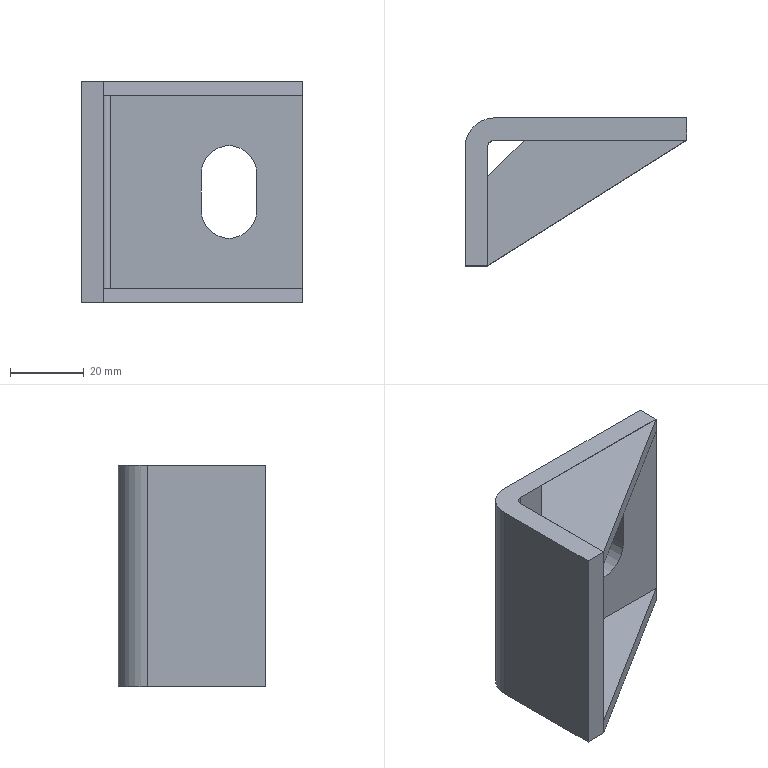Part | STEP file | HL4GZ-1.581.017 (tank top mounting seat weldment) | 3 solids | 26 faces | box 60 x 40 x 60 mm | volume 38051 mm3 | plane 22 | cylinder 4 | commonest cylinder face diameters 15 x2 4 x1 16 x1